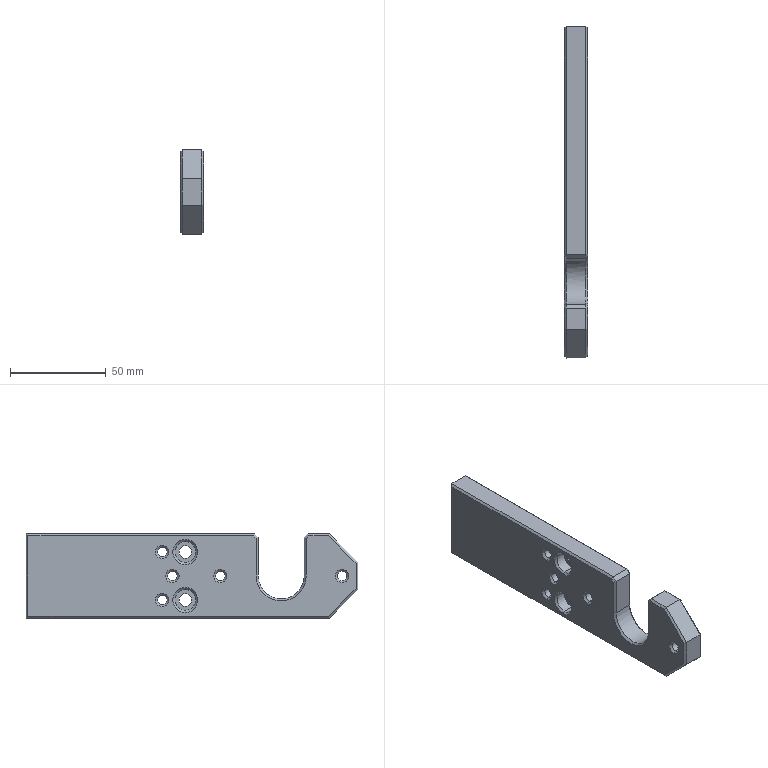Part | SolidWorks | features BaseBody 1 | 1 solid | 87 faces | box 12 x 173 x 44 mm | volume 76150 mm3 | plane 37 | cone 31 | cylinder 19 | commonest cylinder face diameters 5 x10 6.6 x4 11 x4 24 x1